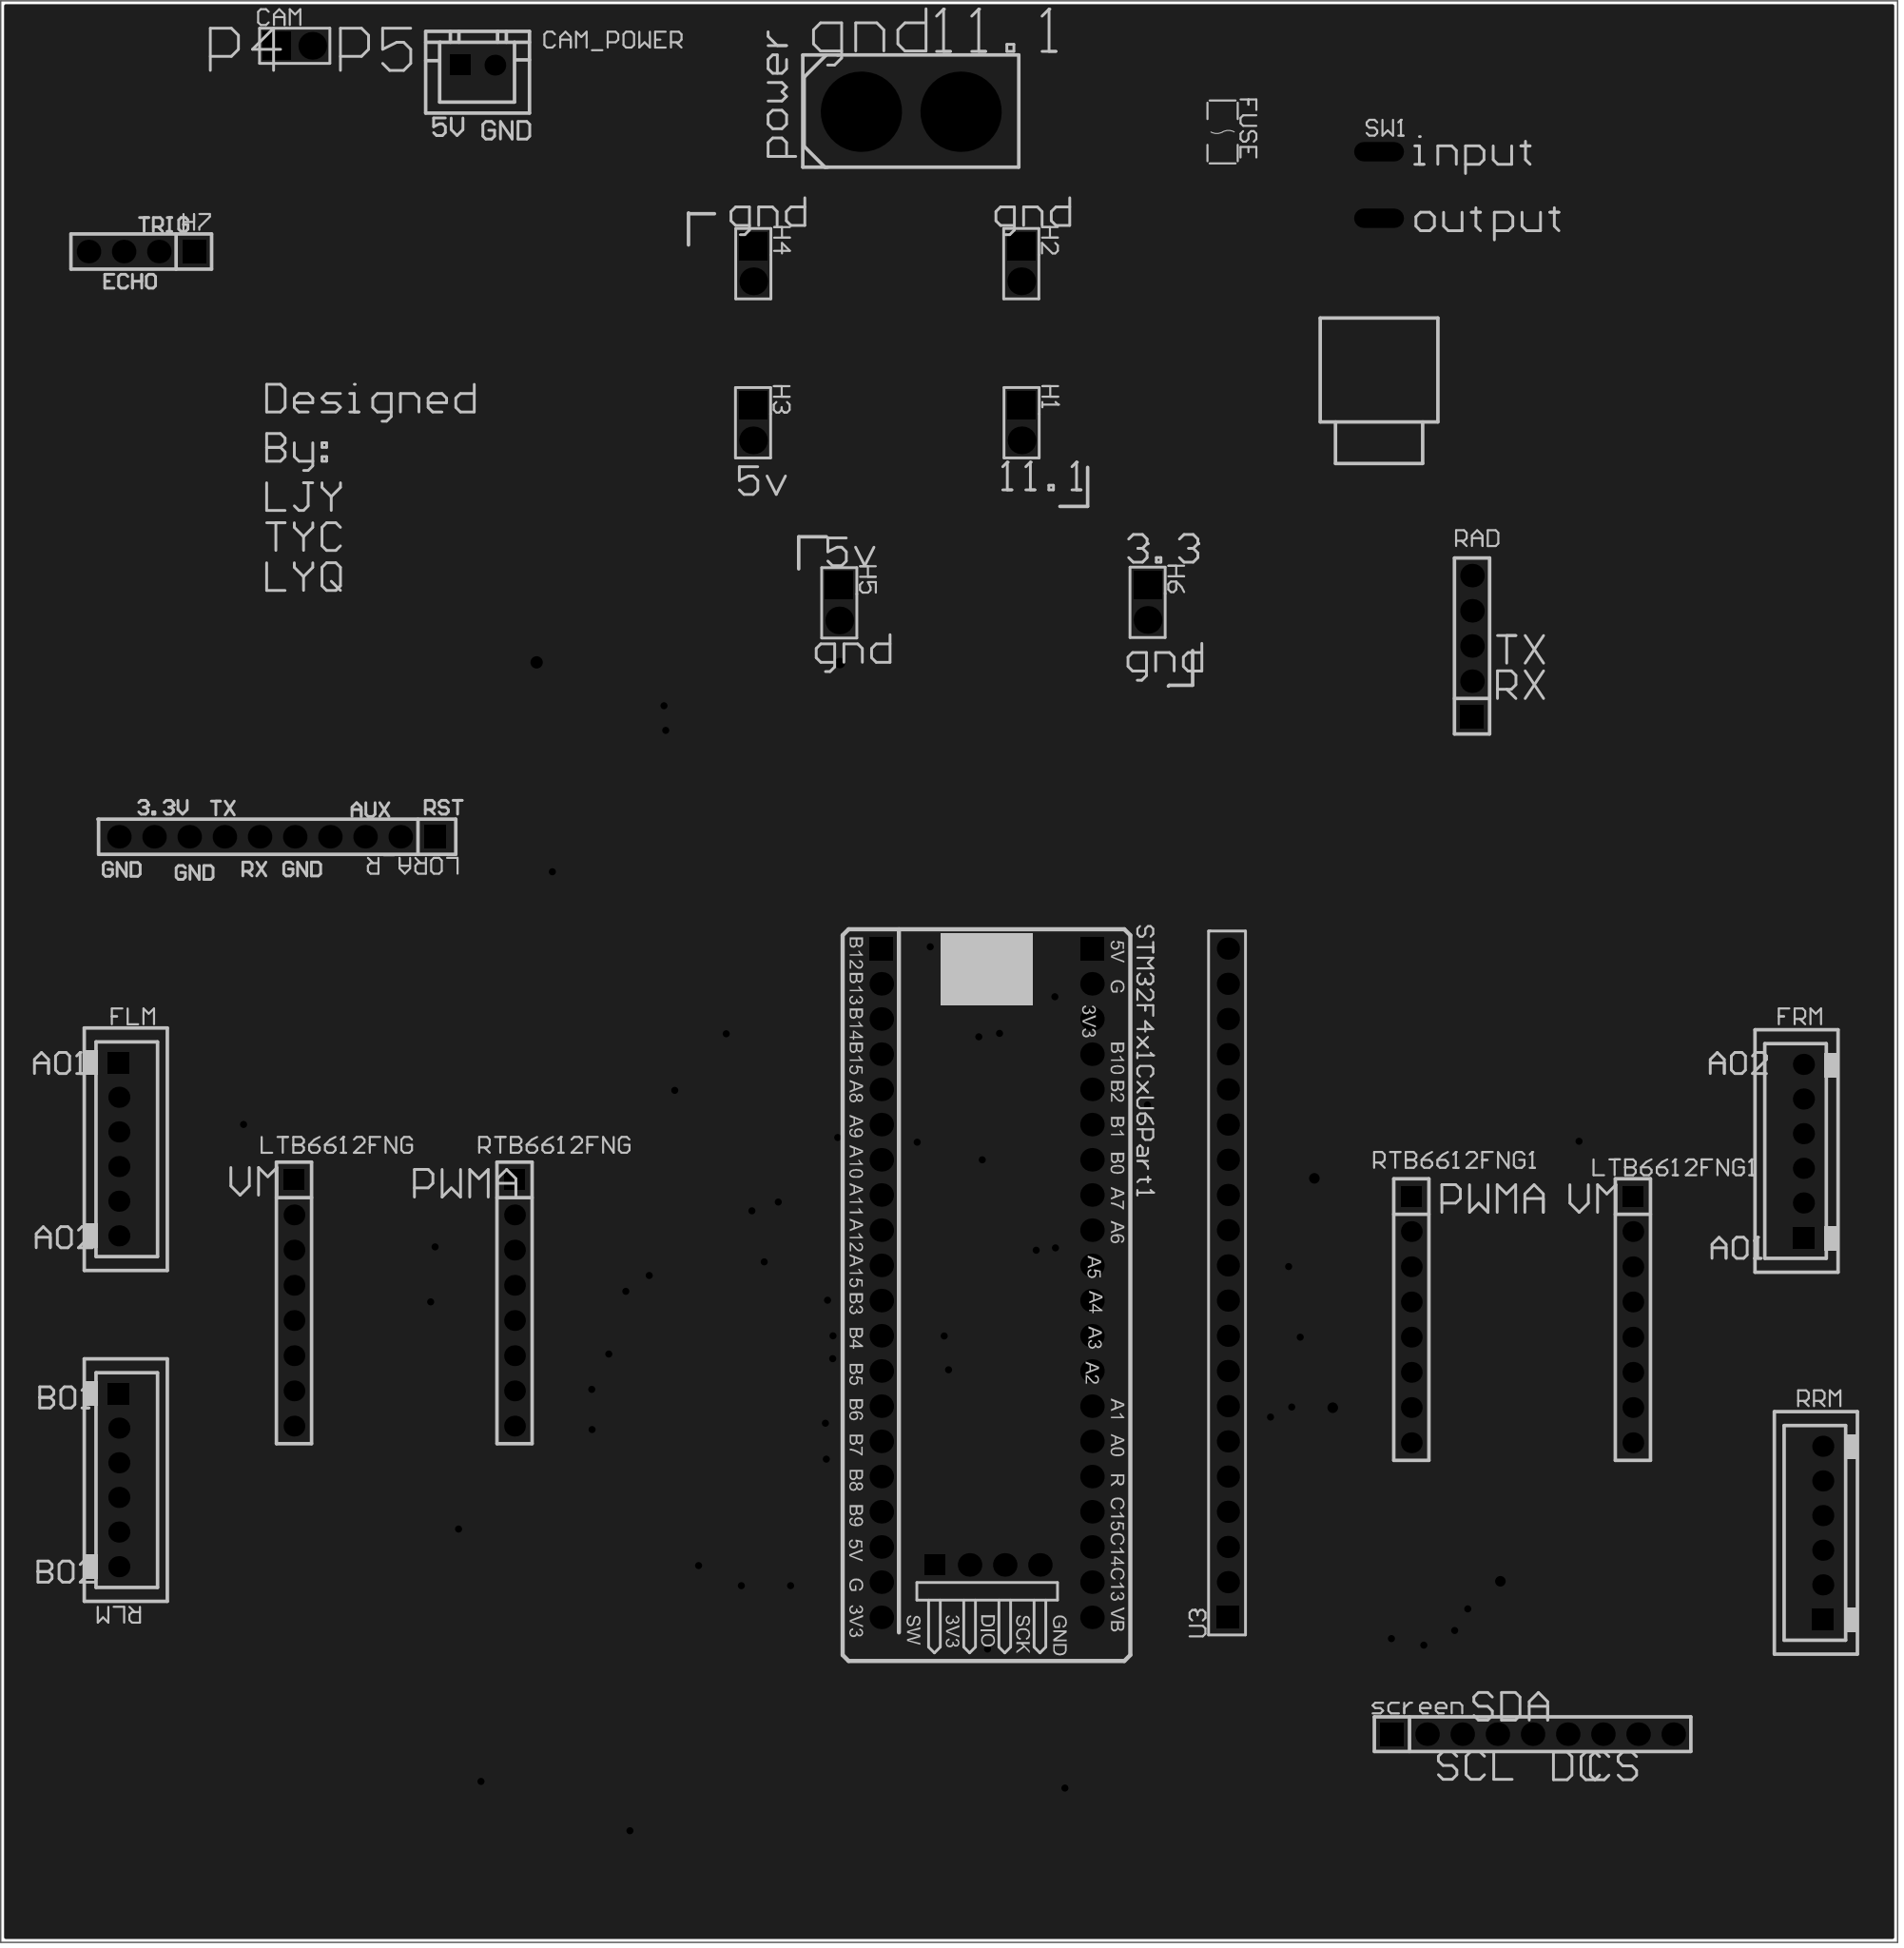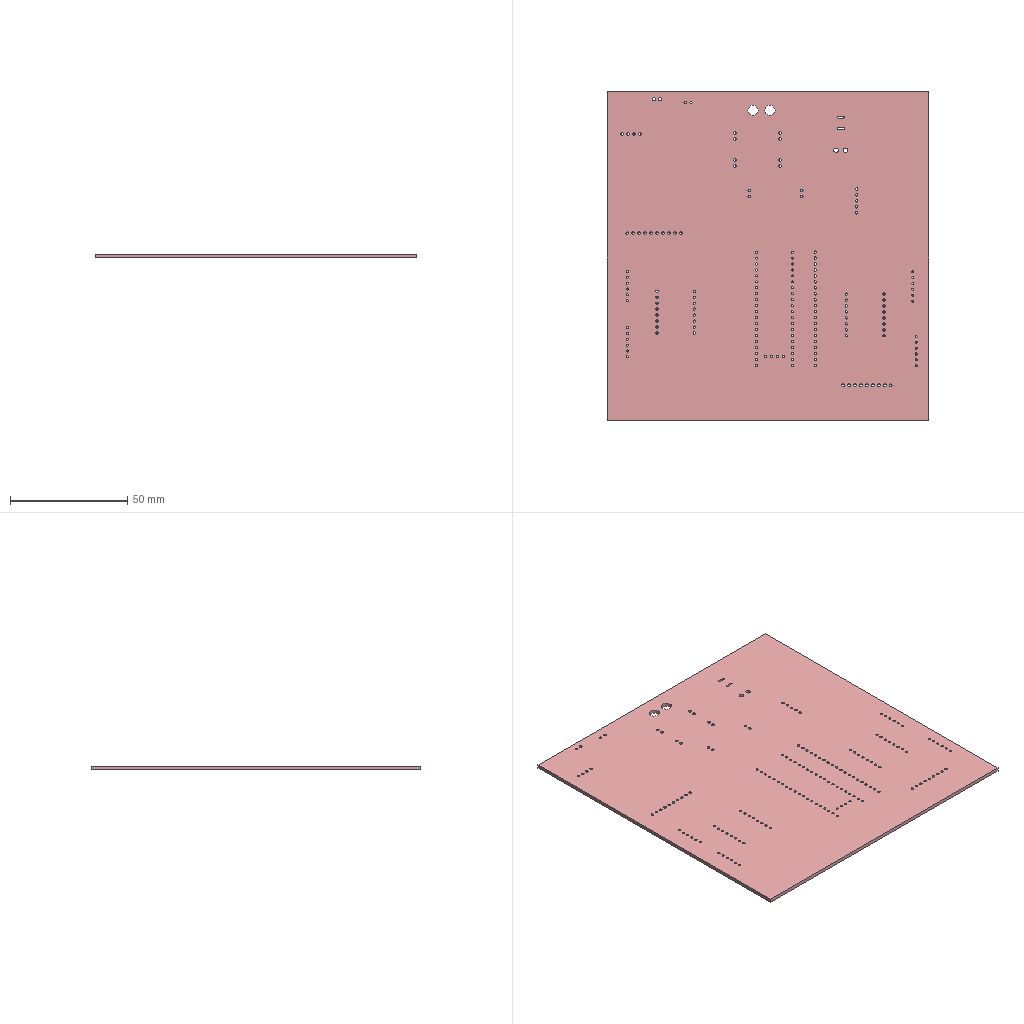Circuit board layout | Altium Designer | box 137 x 140.1 x 1.6 mm
Layer stack:
# Altium Designer layer stack of  (unit mm; dielectric type: 0 none, 1 core, 2 prepreg, 3 surface material)
index,name,kind,layer,copper_thickness_mm,dielectric_type,dielectric_thickness_mm,dielectric_material,dielectric_constant
0,Top Paste Mask Layer,other,,,,,,
1,Top Silkscreen Layer,other,,,,,,
2,Top Solder Mask Layer,dielectric,,,3,0.01,,3.3
3,Top Layer,copper,Top Layer,0.035,,,,
4,Dielectric1,dielectric,,,3,1.51,FR4,4.5
5,Bottom Layer,copper,Bottom Layer,0.035,,,,
6,Bottom Solder Mask Layer,dielectric,,,3,0.01,,3.3
7,Bottom Silkscreen Layer,other,,,,,,
8,Bottom Paste Mask Layer,other,,,,,,
# drill layer pairs: low layer,high layer
drill_pair,Top Layer,Bottom Layer
Part placement:
Designator,Comment,Layer,Footprint,Center-X(mm),Center-Y(mm),Rotation
LTB6612FNG,PZ254V-11-08P,TopLayer,HDR-TH_8P-P2.54-V-M,102.945,125.816,270
RTB6612FNG,PZ254V-11-08P,TopLayer,HDR-TH_8P-P2.54-V-M,118.874,125.816,270
LORA_R,PZ254V-11-10P,TopLayer,HDR-TH_10P-P2.54-V-M,101.731,159.456,180
RAD,PZ254V-11-05P,TopLayer,HDR-TH_5P-P2.54-V-M,188.026,173.222,90
screen,PZ254V-11-09P,TopLayer,HDR-TH_9P-P2.54-V-M,192.401,94.694,0
FUSE,,TopLayer,F1206,170.011,210.317,270
H1,PZ254V-11-02P,TopLayer,HDR-TH_2P-P2.54-V-M,155.495,189.334,270
H2,PZ254V-11-02P,TopLayer,HDR-TH_2P-P2.54-V-M,155.471,200.813,270
H3,PZ254V-11-02P,TopLayer,HDR-TH_2P-P2.54-V-M,136.099,189.332,270
H4,PZ254V-11-02P,TopLayer,HDR-TH_2P-P2.54-V-M,136.119,200.811,270
H5,PZ254V-11-02P,TopLayer,HDR-TH_2P-P2.54-V-M,142.326,176.335,270
H6,PZ254V-11-02P,TopLayer,HDR-TH_2P-P2.54-V-M,164.593,176.373,270
STM32F4x1CxU6Part1,STM32F4x1CxU6 WeActStudio,TopLayer,STM32F4x1CxU6_WeActStudio,152.971,127.254,270
SW1,HX KCD11-BL,TopLayer,SW-TH_KCD11-BL,181.312,206.491,0
U1,XT60-M.,TopLayer,CONN-TH_XT60,147.491,211.776,0
U3,ZX-PZ2.54-1-20PZZ,TopLayer,HDR-TH_20P-P2.54-V-M,170.396,127.254,90
LTB6612FNG1,PZ254V-11-08P,TopLayer,HDR-TH_8P-P2.54-V-M,199.644,124.614,270
RTB6612FNG1,PZ254V-11-08P,TopLayer,HDR-TH_8P-P2.54-V-M,183.642,124.614,270
H7,PZ254V-11-04P,TopLayer,HDR-TH_4P-P2.54-V-M,91.915,201.688,180
CAM_POWER,HX-XH2.54-2PZZ,TopLayer,CONN-TH_2P-P2.50_HX-2.54MM-2P-ZZ-MS,116.205,215.138,0
FLM,HX-XH2.54-6PZZ,TopLayer,CONN-TH_6P-P2.50_BX-XH2.54-6PZZ,90.297,136.906,270
FRM,HX-XH2.54-6PZZ,TopLayer,CONN-TH_6P-P2.50_BX-XH2.54-6PZZ,211.963,136.779,90
CAM,PZ254V-11-02P,TopLayer,HDR-TH_2P-P2.54-V-M,102.997,216.535,0
RLM,HX-XH2.54-6PZZ,TopLayer,CONN-TH_6P-P2.50_BX-XH2.54-6PZZ,90.297,113.03,270
RRM,HX-XH2.54-6PZZ,TopLayer,CONN-TH_6P-P2.50_BX-XH2.54-6PZZ,213.36,109.22,90
Pad and via stacks:
# Altium Designer via and pad stacks of  (unit mm). Each distinct definition once, with the count of objects using it.
# via: kind,start_layer,end_layer,hole_mm,diameter_mm,mode(0 simple;1 top-mid-bottom;2 full stack),diameter_per_layer,count,example_net
# pad: kind,layer,hole_mm,hole_type(0 round;1 square;2 slot),plating,top_size,top_shape(1 round;2 rect;3 octagon;9 rounded rect),mid_size,bottom_size,mode,footprint,size_per_layer,count,example
pad,Multi-Layer,1,0,plated,1.5x1.5,2,1.5x1.5,1.5x1.5,0,HDR-TH_8P-P2.54-V-M,,4,LTB6612FNG.1
pad,Multi-Layer,1,0,plated,1.5x1.5,1,1.5x1.5,1.5x1.5,0,HDR-TH_8P-P2.54-V-M,,28,LTB6612FNG.2
pad,Multi-Layer,1.1,0,plated,1.7x1.7,1,1.7x1.7,1.7x1.7,0,HDR-TH_10P-P2.54-V-M,,9,LORA_R.10
pad,Multi-Layer,1.1,0,plated,1.575x1.7,2,1.575x1.7,1.575x1.7,0,HDR-TH_10P-P2.54-V-M,,1,LORA_R.1
pad,Multi-Layer,1.1,0,plated,1.7x1.7,2,1.7x1.7,1.7x1.7,0,HDR-TH_5P-P2.54-V-M,,1,RAD.1
pad,Multi-Layer,1.1,0,plated,1.7x1.7,1,1.7x1.7,1.7x1.7,0,HDR-TH_5P-P2.54-V-M,,4,RAD.2
pad,Multi-Layer,1.1,0,plated,1.7x1.7,2,1.7x1.7,1.7x1.7,0,HDR-TH_9P-P2.54-V-M,,1,screen.1
pad,Multi-Layer,1.1,0,plated,1.7x1.7,1,1.7x1.7,1.7x1.7,0,HDR-TH_9P-P2.54-V-M,,8,screen.2
pad,Multi-Layer,1.2,0,plated,2x2,2,2x2,2x2,0,HDR-TH_2P-P2.54-V-M,,7,H1.1
pad,Multi-Layer,1.2,0,plated,2x2,1,2x2,2x2,0,HDR-TH_2P-P2.54-V-M,,7,H1.2
pad,Multi-Layer,0.9,0,plated,1.7x1.7,1,1.7x1.7,1.7x1.7,0,STM32F4x1CxU6 WeActStudio,,41,STM32F4x1CxU6Part1.8
pad,Multi-Layer,0.9,0,plated,1.7x1.7,2,1.7x1.7,1.7x1.7,0,STM32F4x1CxU6 WeActStudio,,2,STM32F4x1CxU6Part1.1
pad,Multi-Layer,0.9,0,plated,1.5x1.5,2,1.5x1.5,1.5x1.5,0,STM32F4x1CxU6 WeActStudio,,1,STM32F4x1CxU6Part1.41
pad,Multi-Layer,0.8,2,plated,1.4x3.6,1,1.4x3.6,1.4x3.6,0,SW-TH_KCD11-BL,,2,SW1.1
pad,Multi-Layer,4.4,0,plated,5.8x5.8,1,5.8x5.8,5.8x5.8,0,CONN-TH_XT60,,2,U1.1
pad,Multi-Layer,1.05,0,plated,1.6x1.6,1,1.6x1.6,1.6x1.6,0,HDR-TH_20P-P2.54-V-M,,19,U3.20
pad,Multi-Layer,1.05,0,plated,1.6x1.6,2,1.6x1.6,1.6x1.6,0,HDR-TH_20P-P2.54-V-M,,1,U3.1
pad,Multi-Layer,1.1,0,plated,1.7x1.7,2,1.7x1.7,1.7x1.7,0,HDR-TH_4P-P2.54-V-M,,1,H7.1
pad,Multi-Layer,1.1,0,plated,1.7x1.7,1,1.7x1.7,1.7x1.7,0,HDR-TH_4P-P2.54-V-M,,3,H7.2
pad,Multi-Layer,1,0,plated,1.5x1.5,2,1.5x1.5,1.5x1.5,0,CONN-TH_2P-P2.50_HX-2.54MM-2P-ZZ-MS,,1,CAM_POWER.1
pad,Multi-Layer,1,0,plated,1.5x1.5,1,1.5x1.5,1.5x1.5,0,CONN-TH_2P-P2.50_HX-2.54MM-2P-ZZ-MS,,1,CAM_POWER.2
pad,Multi-Layer,0.9144,0,plated,1.524x1.524,1,1.524x1.524,1.524x1.524,0,CONN-TH_6P-P2.50_BX-XH2.54-6PZZ,,20,FLM.6
pad,Multi-Layer,0.9144,0,plated,1.524x1.524,2,1.524x1.524,1.524x1.524,0,CONN-TH_6P-P2.50_BX-XH2.54-6PZZ,,4,FLM.1
pad,Top Layer,0,0,plated,1.19x1.728,2,1.19x1.728,1.19x1.728,0,F1206,,2,FUSE.1
via,Top Layer,Bottom Layer,0.381,0.762,0,,4,R_PWMB
via,Top Layer,Bottom Layer,0.254,0.508,0,,52,S2_3.3V
via,Top Layer,Bottom Layer,0.381,0.889,0,,1,P_3.3V
Copper pours:
name,layer,net,type(0 solid;1 hatched;2 none)
Bottom Layer-GND,Bottom Layer,GND,0
Top Layer-GND,Top Layer,GND,0
Design rules, without the lines most boards share:
# Altium Designer design rules of  (exported by Altium Designer, unit mm)
# columns: name | kind | enabled | priority | scope1 | scope2 | descriptor | typed fields (field=value)
viaSize | 11 | enabled | 1 | All | All | Routing Via (MinHoleWidth=9mil) (MaxHoleWidth=248.031mil) (PreferredHoleWidth=10mil) (MinWidth=19.685mil) (MaxWidth=393.701mil) (PreferedWidth=20mil) (All) | via_min_hole=0.2286 via_max_hole=6.3 via_preferred_diameter=0.508 via_preferred_hole=0.254
copperRegion_Top Layer | 20 | enabled | 1 | (InNet('GND')) And OnLayer('Top Layer') | All | Polygon Connect Rule(Relief Connect )(Conductor Width=10mil) (Relief Angle=90 Angle) (Entries=4) (Air Gap Width=10mil) ((InNet('GND')) And OnLayer('Top Layer')),(All) | connect_style(0=relief,1=direct,2=none)=0 relief_conductor_width=0.254 relief_entries=4
copperRegion_Bottom Layer | 20 | enabled | 2 | (InNet('GND')) And OnLayer('Bottom Layer') | All | Polygon Connect Rule(Relief Connect )(Conductor Width=10mil) (Relief Angle=90 Angle) (Entries=4) (Air Gap Width=10mil) ((InNet('GND')) And OnLayer('Bottom Layer')),(All) | connect_style(0=relief,1=direct,2=none)=0 relief_conductor_width=0.254 relief_entries=4
copperRegion | 20 | enabled | 3 | (InNet('GND')) | All | Polygon Connect Rule(Direct Connect )(Conductor Width=10mil) (Relief Angle=90 Angle) (Entries=4) (Air Gap Width=10mil) ((InNet('GND'))),(All) | connect_style(0=relief,1=direct,2=none)=1 relief_conductor_width=0.254 relief_entries=4